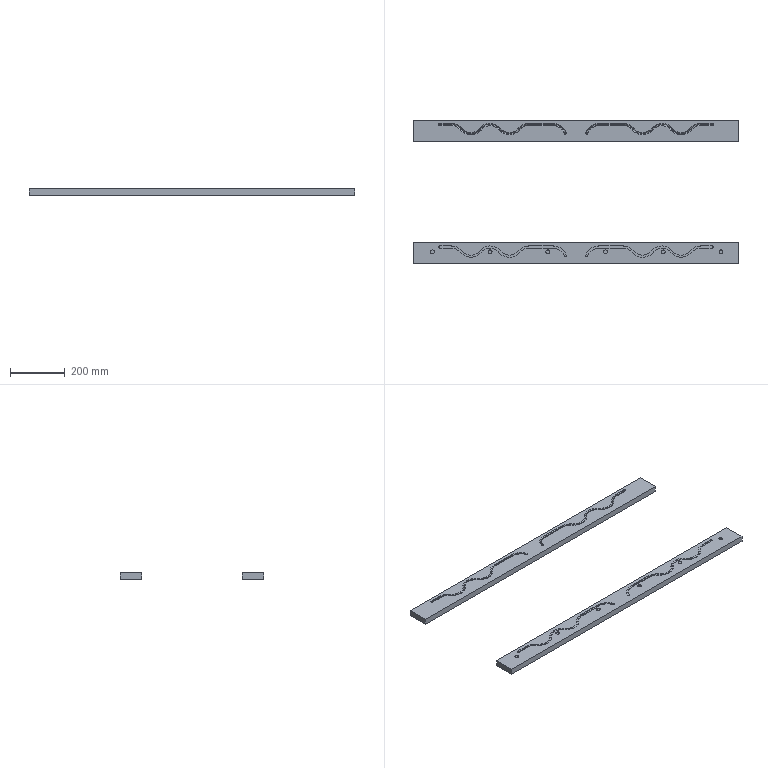Part | 4 solids | 236 faces | box 1185 x 523.484 x 22 mm | volume 8061453 mm3 | torus 120 | cylinder 60 | plane 32 | sphere 12 | cone 12 | commonest cylinder face diameters 4 x48 10.2 x12